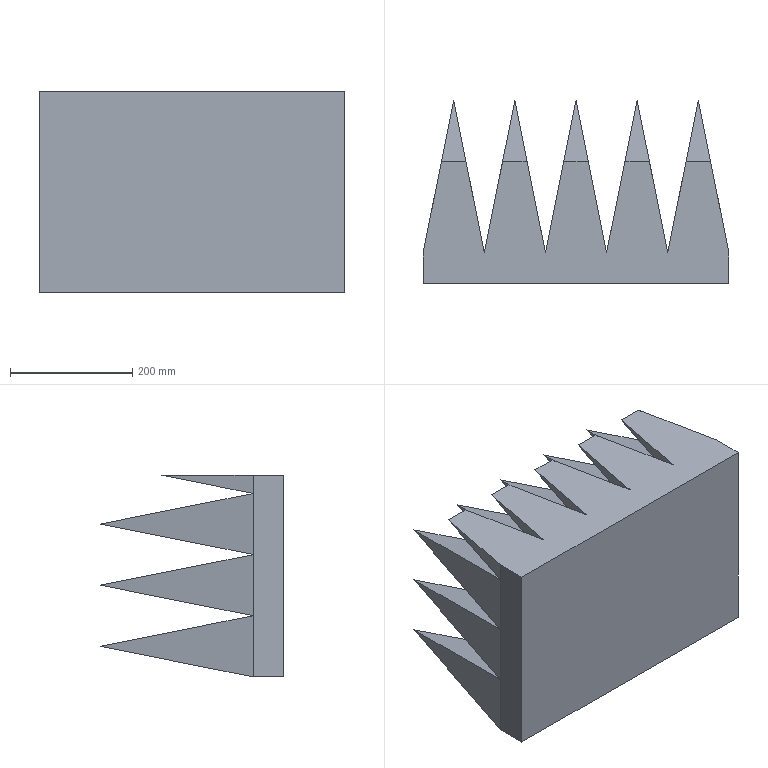Part | SolidWorks | features LPattern 2, Blend 1, Extrusion 1, ICE 1 | 1 solid | 80 faces | box 500 x 300 x 330 mm | volume 21650000 mm3 | plane 80